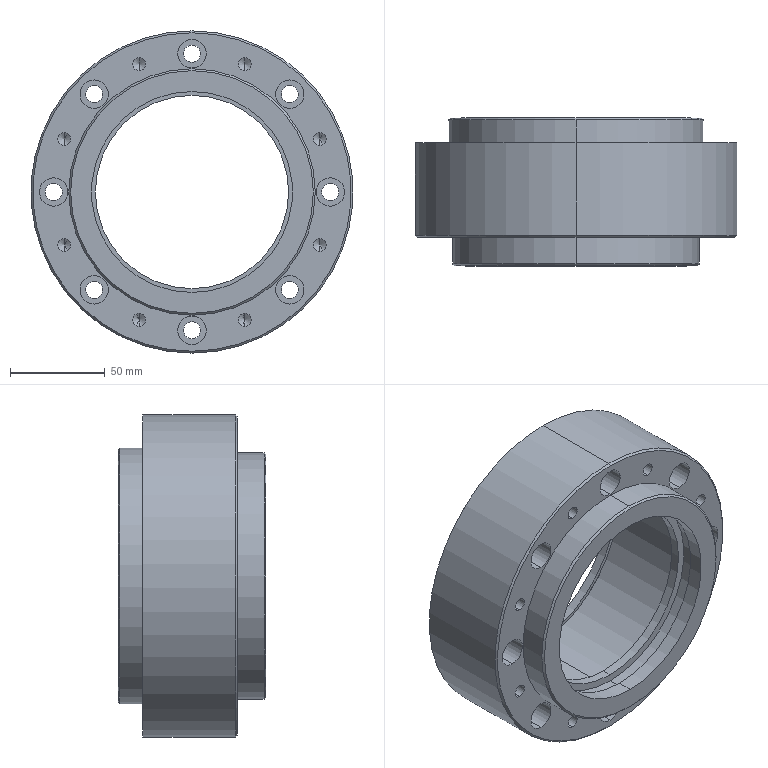Part | SolidWorks | features ICE 15, Chamfer 3, CirPattern 3, HoleWzd 3, Extrusion 1 | 1 solid | 105 faces | box 170 x 78 x 170 mm | volume 615518 mm3 | cylinder 66 | cone 22 | plane 17 | commonest cylinder face diameters 6.8 x16 9 x16 15 x16 102 x2 106 x2 110 x2